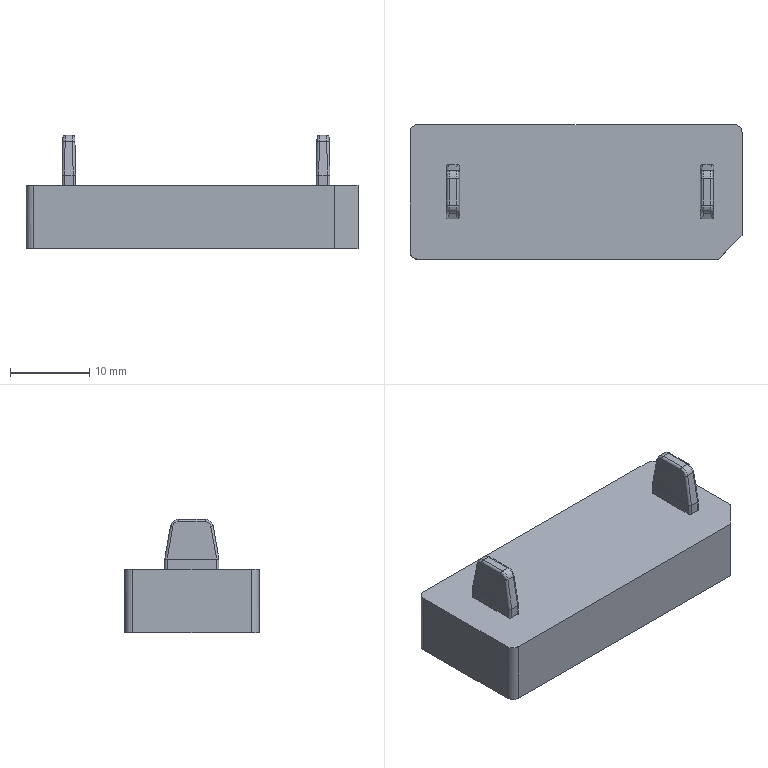NC program | PowerMill | posted by the shop | part box 42 x 17 x 14.346 mm
Lines 32786 to 34275 of 86217:
( TOOL ID   B4R0.5_1_1 )
( TOOL DIA. 4. TIP RAD .5 LENGTH 61.52 )
( Z = -6.52 )
T5 M6
T13
G91 G28 Z0
G0 G90 G54
M08
S18000 M3
X0 Y0 M8
G43 Z10.796 H5
X18.342 Y-3.827
Z.917
G1 Z-.283 F1200
X18.325 Y-3.779 F2000
X18.304 Y-3.733
X18.28 Y-3.689
X18.253 Y-3.646
X18.222 Y-3.606
X18.188 Y-3.569
X18.151 Y-3.534
X18.112 Y-3.503
X18.07 Y-3.474
X18.026 Y-3.449
X17.98 Y-3.427
X17.933 Y-3.41
X17.885 Y-3.396
X17.835 Y-3.385
X17.785 Y-3.379
X17.734 Y-3.377
X17.684 Y-3.378
X17.634 Y-3.384
X17.584 Y-3.394
X17.541 Y-3.406
X17.486 Y-3.423
X17.429 Y-3.438
X17.373 Y-3.451
X17.316 Y-3.462
X17.255 Y-3.471
X17.194 Y-3.478
X17.133 Y-3.483
X17.07 Y-3.486
X17.008 Y-3.487
X16.947
X16.885 Y-3.486
X16.823
X16.631
X16.509 Y-3.487
X16.405 Y-3.486
X16.291
X16.047 Y-3.485
X16.009 Y-3.483
X15.972 Y-3.479
X15.924 Y-3.474
X15.887 Y-3.469
X15.849 Y-3.463
X15.812 Y-3.456
X15.743 Y-3.441
X15.69 Y-3.427
X15.61 Y-3.403
X15.53 Y-3.373
X15.451 Y-3.341
X15.377 Y-3.306
X15.307 Y-3.269
X15.243 Y-3.231
X15.184 Y-3.192
X15.13 Y-3.153
X15.077 Y-3.112
X15.025 Y-3.07
X14.975 Y-3.025
X14.928 Y-2.979
X14.883 Y-2.93
X14.839 Y-2.879
X14.798 Y-2.827
X14.758 Y-2.773
X14.711 Y-2.706
X14.668 Y-2.636
X14.628 Y-2.565
X14.591 Y-2.491
X14.558 Y-2.416
X14.528 Y-2.338
X14.501 Y-2.257
X14.477 Y-2.174
X14.457 Y-2.088
X14.44 Y-1.999
X14.429 Y-1.93
X14.421 Y-1.86
X14.417 Y-1.78
X14.414 Y-1.685
Y-1.558
Y1.194
Y1.558
Y1.623
Y1.688
X14.415 Y1.752
X14.417 Y1.821
X14.422 Y1.9
X14.429 Y1.972
X14.438 Y2.036
X14.45 Y2.099
X14.464 Y2.162
X14.48 Y2.224
X14.498 Y2.286
X14.519 Y2.351
X14.542 Y2.416
X14.568 Y2.479
X14.597 Y2.541
X14.628 Y2.602
X14.66 Y2.662
X14.695 Y2.721
X14.736 Y2.784
X14.782 Y2.847
X14.834 Y2.912
X14.892 Y2.978
X14.947 Y3.036
X15.006 Y3.091
X15.068 Y3.144
X15.132 Y3.195
X15.2 Y3.242
X15.271 Y3.287
X15.345 Y3.329
X15.412 Y3.363
X15.483 Y3.395
X15.558 Y3.424
X15.637 Y3.45
X15.72 Y3.474
X15.809 Y3.495
X15.872 Y3.507
X15.94 Y3.516
X16.015 Y3.522
X16.1 Y3.525
X16.164 Y3.526
X16.509 Y3.525
X16.727 Y3.524
X16.97 Y3.525
X17.068
X17.144 Y3.522
X17.201 Y3.517
X17.252 Y3.511
X17.304 Y3.503
X17.354 Y3.494
X17.405 Y3.483
X17.455 Y3.47
X17.525 Y3.449
X17.595 Y3.426
X17.664 Y3.4
X17.731 Y3.372
X17.799 Y3.338
X17.869 Y3.299
X17.939 Y3.256
X18.009 Y3.209
X18.075 Y3.159
X18.137 Y3.108
X18.191 Y3.058
X18.243 Y3.006
X18.296 Y2.947
X18.352 Y2.88
X18.392 Y2.829
X18.427 Y2.779
X18.461 Y2.727
X18.492 Y2.674
X18.526 Y2.613
X18.563 Y2.54
X18.599 Y2.461
X18.628 Y2.39
X18.65 Y2.328
X18.668 Y2.269
X18.684 Y2.209
X18.705 Y2.115
X18.722 Y2.029
X18.733 Y1.95
X18.741 Y1.873
X18.745 Y1.792
X18.746 Y1.693
Y1.558
Y-.169
Y-1.443
X18.747 Y-1.607
X18.746 Y-1.72
X18.742 Y-1.813
X18.736 Y-1.894
X18.728 Y-1.961
X18.716 Y-2.028
X18.701 Y-2.102
X18.68 Y-2.184
X18.654 Y-2.271
X18.626 Y-2.353
X18.597 Y-2.427
X18.568 Y-2.493
X18.538 Y-2.554
X18.505 Y-2.613
X18.457 Y-2.692
X18.409 Y-2.764
X18.36 Y-2.831
X18.31 Y-2.892
X18.26 Y-2.949
X18.207 Y-3.002
X18.144 Y-3.061
X18.081 Y-3.114
X18.018 Y-3.163
X17.955 Y-3.207
X17.891 Y-3.246
X17.815 Y-3.289
X17.738 Y-3.327
X17.66 Y-3.361
X17.581 Y-3.392
X17.541 Y-3.406
X17.476 Y-3.427 Z-.284
X17.407 Y-3.445
X17.334 Y-3.461
X17.269 Y-3.472
X17.202 Y-3.481
X17.137 Y-3.487
X17.072 Y-3.49
X16.924 Y-3.491
X16.63 Y-3.492 Z-.285
X16.393 Y-3.495
X16.214 Y-3.496 Z-.286
X16.045 Y-3.494
X15.977 Y-3.491
X15.907 Y-3.484
X15.834 Y-3.473
X15.758 Y-3.458
X15.679 Y-3.438 Z-.287
X15.599 Y-3.413
X15.52 Y-3.386
X15.444 Y-3.354
X15.37 Y-3.32
X15.298 Y-3.282
X15.227 Y-3.24 Z-.288
X15.166 Y-3.2
X15.108 Y-3.159
X15.052 Y-3.114
X14.992 Y-3.062
X14.931 Y-3.005
X14.88 Y-2.952
X14.832 Y-2.899 Z-.289
X14.787 Y-2.844
X14.735 Y-2.775
X14.687 Y-2.704
X14.643 Y-2.631
X14.602 Y-2.557 Z-.29
X14.565 Y-2.482
X14.532 Y-2.406
X14.508 Y-2.344
X14.486 Y-2.281
X14.466 Y-2.218
X14.449 Y-2.154 Z-.291
X14.434 Y-2.089
X14.421 Y-2.024
X14.41 Y-1.959
X14.399 Y-1.879
X14.392 Y-1.798 Z-.292
X14.389 Y-1.715
Y-1.631
X14.382 Y-.215 Z-.295
X14.374 Y1.283 Z-.298
X14.372 Y1.617
Y1.741 Z-.299
X14.373 Y1.83
X14.378 Y1.904
X14.387 Y1.989
X14.4 Y2.074
X14.417 Y2.161
X14.439 Y2.249 Z-.3
X14.465 Y2.338
X14.492 Y2.419
X14.522 Y2.496
X14.554 Y2.57
X14.589 Y2.64
X14.63 Y2.713
X14.675 Y2.787
X14.724 Y2.859 Z-.301
X14.775 Y2.928
X14.827 Y2.992
X14.88 Y3.05
X14.933 Y3.104
X14.985 Y3.153
X15.04 Y3.2
X15.096 Y3.245
X15.154 Y3.288
X15.214 Y3.328
X15.282 Y3.369 Z-.302
X15.352 Y3.407
X15.425 Y3.443
X15.5 Y3.475
X15.578 Y3.504
X15.659 Y3.53
X15.727 Y3.549
X15.795 Y3.565 Z-.303
X15.863 Y3.579
X15.932 Y3.589
X16.002 Y3.596
X16.072 Y3.6
X16.142 Y3.601
X16.212
X16.52 Y3.603 Z-.304
X16.827 Y3.606 Z-.305
X17.087 Y3.607
X17.15 Y3.605
X17.219 Y3.599
X17.293 Y3.589 Z-.306
X17.375 Y3.574
X17.449 Y3.558
X17.524 Y3.537
X17.601 Y3.512
X17.681 Y3.483 Z-.307
X17.759 Y3.45
X17.823 Y3.419
X17.887 Y3.384
X17.955 Y3.344
X18.025 Y3.297 Z-.308
X18.094 Y3.247
X18.158 Y3.196
X18.214 Y3.147
X18.266 Y3.097 Z-.309
X18.324 Y3.036
X18.38 Y2.972
X18.432 Y2.906
X18.481 Y2.838
X18.527 Y2.767 Z-.31
X18.569 Y2.694
X18.612 Y2.614
X18.649 Y2.534
X18.682 Y2.455
X18.711 Y2.377 Z-.311
X18.736 Y2.297
X18.759 Y2.211
X18.779 Y2.122
X18.795 Y2.031
X18.807 Y1.939
X18.815 Y1.844 Z-.312
X18.82 Y1.748
X18.821 Y1.65
X18.822 Y1.154 Z-.313
X18.826 Y.432 Z-.314
X18.828 Y-.229 Z-.316
X18.834 Y-1.559 Z-.318
X18.835 Y-1.642 Z-.319
X18.833 Y-1.752
X18.829 Y-1.843
X18.822 Y-1.926
X18.81 Y-2.016
X18.794 Y-2.105
X18.774 Y-2.194 Z-.32
X18.751 Y-2.281
X18.724 Y-2.367
X18.693 Y-2.451
X18.658 Y-2.534
X18.62 Y-2.615 Z-.321
X18.579 Y-2.693
X18.534 Y-2.769
X18.486 Y-2.843
X18.445 Y-2.901
X18.401 Y-2.957
X18.351 Y-3.017 Z-.322
X18.293 Y-3.079
X18.23 Y-3.142
X18.169 Y-3.198
X18.11 Y-3.247
X18.053 Y-3.29
X17.996 Y-3.329
X17.922 Y-3.376 Z-.323
X17.847 Y-3.419
X17.775 Y-3.456
X17.705 Y-3.487
X17.638 Y-3.514
X17.582 Y-3.532
X17.508 Y-3.557 Z-.324
X17.431 Y-3.579
X17.353 Y-3.596
X17.276 Y-3.61
X17.201 Y-3.619
X17.129 Y-3.625
X17.058 Y-3.626
X16.967 Y-3.627 Z-.325
X16.875 Y-3.628
X16.784 Y-3.629
X16.693 Y-3.63
X16.566 Y-3.631
X16.475 Y-3.632
X16.384 Z-.326
X16.293 Y-3.633
X16.202
X16.111 Y-3.632
X16.036 Y-3.631
X15.961 Y-3.626
X15.887 Y-3.618 Z-.327
X15.811 Y-3.606
X15.733 Y-3.589
X15.653 Y-3.568
X15.569 Y-3.542
X15.498 Y-3.517
X15.426 Y-3.488 Z-.328
X15.353 Y-3.454
X15.283 Y-3.418
X15.217 Y-3.381
X15.152 Y-3.34
X15.086 Y-3.294
X15.02 Y-3.243 Z-.329
X14.952 Y-3.186
X14.894 Y-3.133
X14.838 Y-3.076
X14.782 Y-3.014
X14.727 Y-2.948
X14.675 Y-2.878 Z-.33
X14.625 Y-2.805
X14.578 Y-2.729
X14.536 Y-2.654
X14.498 Y-2.579
X14.465 Y-2.505
X14.436 Y-2.431
X14.412 Y-2.366 Z-.331
X14.391 Y-2.301
X14.366 Y-2.211
X14.346 Y-2.129
X14.331 Y-2.052
X14.32 Y-1.978
X14.311 Y-1.894 Z-.332
X14.304 Y-1.81
X14.301 Y-1.726
X14.299 Y-1.642
Y-1.557
Y-1.473
X14.296 Y-.71 Z-.334
X14.292 Y.46 Z-.336
X14.287 Y1.623 Z-.338
Y1.698
X14.289 Y1.806 Z-.339
X14.293 Y1.894
X14.299 Y1.972
X14.309 Y2.046
X14.326 Y2.143
X14.346 Y2.237 Z-.34
X14.37 Y2.328
X14.396 Y2.414
X14.426 Y2.498
X14.46 Y2.581
X14.497 Y2.663
X14.538 Y2.742 Z-.341
X14.582 Y2.82
X14.629 Y2.895
X14.68 Y2.968
X14.734 Y3.039
X14.792 Y3.107
X14.84 Y3.16 Z-.342
X14.89 Y3.21
X14.947 Y3.262
X15.013 Y3.318
X15.071 Y3.363
X15.128 Y3.405
X15.188 Y3.444
X15.26 Y3.487 Z-.343
X15.335 Y3.527
X15.411 Y3.563
X15.49 Y3.597
X15.571 Y3.626
X15.653 Y3.652
X15.737 Y3.674 Z-.344
X15.818 Y3.692
X15.895 Y3.706
X15.967 Y3.715
X16.036 Y3.719
X16.104 Y3.721
X16.197 Y3.722
X16.29 Y3.723 Z-.345
X16.382 Y3.724
X16.475
X16.596 Y3.725
X16.688
X16.781 Z-.346
X16.874
X16.966
X17.059
X17.126
X17.195 Y3.72
X17.268 Y3.712 Z-.347
X17.345 Y3.699
X17.428 Y3.681
X17.52 Y3.657
X17.587 Y3.638
X17.656 Y3.614
X17.729 Y3.584
X17.806 Y3.55 Z-.348
X17.883 Y3.511
X17.957 Y3.469
X18.025 Y3.426
X18.086 Y3.384
X18.144 Y3.339
X18.209 Y3.286 Z-.349
X18.272 Y3.228
X18.335 Y3.166
X18.395 Y3.101
X18.451 Y3.034
X18.503 Y2.967
X18.55 Y2.9 Z-.35
X18.593 Y2.83
X18.638 Y2.753
X18.679 Y2.672
X18.718 Y2.589
X18.753 Y2.502
X18.783 Y2.42 Z-.351
X18.81 Y2.336
X18.833 Y2.249
X18.852 Y2.16
X18.869 Y2.067
X18.881 Y1.973
X18.89 Y1.875 Z-.352
X18.896 Y1.774
X18.898 Y1.674
X18.899 Y1.011 Z-.353
X18.902 Y.067 Z-.355
X18.905 Y-.823 Z-.357
X18.908 Y-1.675 Z-.359
X18.906 Y-1.772
X18.9 Y-1.869
X18.891 Y-1.964
X18.878 Y-2.059
X18.86 Y-2.152
X18.84 Y-2.243 Z-.36
X18.815 Y-2.332
X18.787 Y-2.42
X18.755 Y-2.506
X18.72 Y-2.591
X18.681 Y-2.673 Z-.361
X18.639 Y-2.753
X18.594 Y-2.831
X18.546 Y-2.906
X18.494 Y-2.979
X18.44 Y-3.048
X18.384 Y-3.114 Z-.362
X18.325 Y-3.177
X18.263 Y-3.237
X18.198 Y-3.295
X18.131 Y-3.349
X18.061 Y-3.4
X17.99 Y-3.448 Z-.363
X17.916 Y-3.492
X17.841 Y-3.532
X17.765 Y-3.569
X17.687 Y-3.602
X17.616 Y-3.628
X17.53 Y-3.656 Z-.364
X17.447 Y-3.679
X17.367 Y-3.698
X17.292 Y-3.711
X17.215 Y-3.721
X17.133 Y-3.728
X17.044 Y-3.731
X16.947 Z-.365
X16.751
X16.484 Y-3.733 Z-.366
X16.196 Y-3.735
X16.117
X16.038 Y-3.733
X15.96 Y-3.727 Z-.367
X15.88 Y-3.718
X15.8 Y-3.705
X15.723 Y-3.689
X15.646 Y-3.669
X15.571 Y-3.646
X15.492 Y-3.619
X15.414 Y-3.588 Z-.368
X15.338 Y-3.554
X15.265 Y-3.516
X15.195 Y-3.476
X15.126 Y-3.433
X15.057 Y-3.386
X14.991 Y-3.335 Z-.369
X14.926 Y-3.281
X14.864 Y-3.225
X14.805 Y-3.166
X14.759 Y-3.117
X14.715 Y-3.066
X14.673 Y-3.013
X14.627 Y-2.95 Z-.37
X14.577 Y-2.877
X14.539 Y-2.817
X14.504 Y-2.759
X14.472 Y-2.699
X14.433 Y-2.616
X14.396 Y-2.532
X14.363 Y-2.446 Z-.371
X14.334 Y-2.358
X14.308 Y-2.269
X14.286 Y-2.178
X14.268 Y-2.086
X14.253 Y-1.993
X14.242 Y-1.898 Z-.372
X14.235 Y-1.801
X14.232 Y-1.703
Y-1.603
X14.228 Y-.402 Z-.374
X14.226 Y.785 Z-.377
X14.223 Y1.51 Z-.378
X14.222 Y1.674
X14.223 Y1.771 Z-.379
X14.227 Y1.874
X14.235 Y1.974
X14.247 Y2.069
X14.261 Y2.158
X14.278 Y2.242
X14.299 Y2.325 Z-.38
X14.325 Y2.417
X14.355 Y2.505
X14.387 Y2.592
X14.423 Y2.675
X14.463 Y2.757
X14.505 Y2.836 Z-.381
X14.551 Y2.914
X14.6 Y2.988
X14.652 Y3.06
X14.707 Y3.13
X14.765 Y3.196
X14.825 Y3.26 Z-.382
X14.888 Y3.321
X14.953 Y3.378
X15.021 Y3.433
X15.091 Y3.484
X15.163 Y3.531
X15.236 Y3.575 Z-.383
X15.312 Y3.615
X15.388 Y3.651
X15.466 Y3.685
X15.548 Y3.714
X15.631 Y3.741
X15.715 Y3.763 Z-.384
X15.8 Y3.782
X15.885 Y3.797
X15.969 Y3.807
X16.052 Y3.814
X16.134 Y3.816
X16.215 Y3.815 Z-.385
X16.502 Y3.814
X16.79 Y3.816 Z-.386
X17.007 Y3.818
X17.095 Y3.817
X17.18 Y3.813
X17.261 Y3.805 Z-.387
X17.34 Y3.793
X17.416 Y3.778
X17.491 Y3.759
X17.578 Y3.734
X17.662 Y3.705
X17.745 Y3.673
X17.814 Y3.642 Z-.388
X17.882 Y3.609
X17.952 Y3.57
X18.026 Y3.524
X18.1 Y3.475
X18.167 Y3.426
X18.226 Y3.379 Z-.389
X18.283 Y3.329
X18.345 Y3.269
X18.405 Y3.206
X18.463 Y3.139
X18.519 Y3.069
X18.572 Y2.995 Z-.39
X18.622 Y2.919
X18.669 Y2.841
X18.713 Y2.761
X18.752 Y2.68
X18.787 Y2.598
X18.821 Y2.51 Z-.391
X18.851 Y2.42
X18.877 Y2.329
X18.9 Y2.236
X18.919 Y2.142
X18.934 Y2.046
X18.945 Y1.956 Z-.392
X18.952 Y1.861
X18.956 Y1.757
X18.957 Y1.642
X18.959 Y.667 Z-.394
X18.964 Y-1.001 Z-.397
X18.966 Y-1.676 Z-.398
X18.964 Y-1.774 Z-.399
X18.959 Y-1.873
X18.949 Y-1.972
X18.936 Y-2.069
X18.918 Y-2.166
X18.898 Y-2.26 Z-.4
X18.873 Y-2.352
X18.845 Y-2.442
X18.814 Y-2.529
X18.78 Y-2.614
X18.741 Y-2.699
X18.699 Y-2.782 Z-.401
X18.654 Y-2.862
X18.607 Y-2.939
X18.556 Y-3.013
X18.502 Y-3.084
X18.446 Y-3.153
X18.387 Y-3.218 Z-.402
X18.325 Y-3.282
X18.259 Y-3.342
X18.196 Y-3.396
X18.129 Y-3.448
X18.058 Y-3.498
X17.985 Y-3.545 Z-.403
X17.91 Y-3.588
X17.834 Y-3.627
X17.759 Y-3.661
X17.685 Y-3.691
X17.641 Y-3.707
X17.552 Y-3.736 Z-.404
X17.467 Y-3.76
X17.388 Y-3.78
X17.311 Y-3.795
X17.238 Y-3.805
X17.165 Y-3.811
X17.093 Y-3.814
X17.02 Y-3.815 Z-.405
X16.636 Y-3.816
X16.252 Y-3.818 Z-.406
X16.162 Y-3.819
X16.086
X16.01 Y-3.816
X15.934 Y-3.81 Z-.407
X15.859 Y-3.8
X15.784 Y-3.787
X15.704 Y-3.769
X15.63 Y-3.749
X15.557 Y-3.728
X15.476 Y-3.7
X15.397 Y-3.669 Z-.408
X15.321 Y-3.634
X15.247 Y-3.597
X15.176 Y-3.556
X15.107 Y-3.512
X15.032 Y-3.461
X14.961 Y-3.407
X14.893 Y-3.35 Z-.409
X14.828 Y-3.291
X14.767 Y-3.23
X14.71 Y-3.167
X14.653 Y-3.098
X14.598 Y-3.027
X14.547 Y-2.953 Z-.41
X14.498 Y-2.876
X14.453 Y-2.796
X14.41 Y-2.714
X14.371 Y-2.63
X14.336 Y-2.543
X14.303 Y-2.454 Z-.411
X14.275 Y-2.364
X14.249 Y-2.271
X14.228 Y-2.177
X14.21 Y-2.081
X14.196 Y-1.983 Z-.412
X14.186 Y-1.884
X14.179 Y-1.783
X14.177 Y-1.681
Y-1.578
X14.173 Y.002 Z-.415
X14.171 Y1.24 Z-.418
X14.17 Y1.674
X14.171 Y1.785 Z-.419
X14.176 Y1.891
X14.184 Y1.992
X14.196 Y2.09
X14.212 Y2.184
X14.23 Y2.277
X14.252 Y2.366 Z-.42
X14.279 Y2.459
X14.309 Y2.548
X14.342 Y2.636
X14.379 Y2.721
X14.419 Y2.804
X14.462 Y2.884 Z-.421
X14.508 Y2.963
X14.558 Y3.039
X14.609 Y3.111
X14.664 Y3.182
X14.722 Y3.25
X14.784 Y3.316 Z-.422
X14.848 Y3.378
X14.914 Y3.438
X14.982 Y3.493
X15.046 Y3.541
X15.116 Y3.589
X15.19 Y3.635 Z-.423
X15.266 Y3.677
X15.34 Y3.713
X15.411 Y3.745
X15.482 Y3.772
X15.547 Y3.794
X15.612 Y3.815
X15.678 Y3.833 Z-.424
X15.708 Y3.842
X15.737 Y3.849
X15.767 Y3.855
X15.802 Y3.862
X15.85 Y3.871
X15.88 Y3.876
X15.91 Y3.88
X15.94 Y3.884
X16.03 Y3.889
X16.134 Y3.892
X16.273 Y3.893 Z-.425
X16.555 Y3.894
X16.97 Y3.896 Z-.426
X17.038
X17.106 Y3.895
X17.174 Y3.892
X17.242 Y3.886
X17.31 Y3.877 Z-.427
X17.377 Y3.864
X17.443 Y3.849
X17.509 Y3.832
X17.575 Y3.814
X17.652 Y3.79
X17.73 Y3.76
X17.809 Y3.726 Z-.428
X17.882 Y3.691
X17.959 Y3.65
X18.033 Y3.606
X18.105 Y3.559
X18.174 Y3.509
X18.241 Y3.456 Z-.429
X18.309 Y3.396
X18.374 Y3.334
X18.435 Y3.27
X18.493 Y3.204
X18.548 Y3.136
X18.599 Y3.066
X18.65 Y2.989 Z-.43
X18.698 Y2.911
X18.742 Y2.831
X18.783 Y2.748
X18.821 Y2.664
X18.855 Y2.577 Z-.431
X18.886 Y2.488
X18.914 Y2.398
X18.938 Y2.305
X18.959 Y2.21
X18.976 Y2.113
X18.989 Y2.013 Z-.432
X18.999 Y1.911
X19.005 Y1.807
X19.008 Y1.7
X19.007 Y1.589
Y1.07 Z-.433
X19.01 Y.304 Z-.435
Y-.368 Z-.436
X19.013 Y-1.297 Z-.438
X19.014 Y-1.559
Y-1.697
X19.011 Y-1.806 Z-.439
X19.005 Y-1.899
X18.996 Y-1.992
X18.983 Y-2.091
X18.965 Y-2.188
X18.944 Y-2.285 Z-.44
X18.919 Y-2.379
X18.89 Y-2.472
X18.858 Y-2.563
X18.823 Y-2.652
X18.784 Y-2.738
X18.742 Y-2.822 Z-.441
X18.697 Y-2.903
X18.649 Y-2.982
X18.598 Y-3.057
X18.544 Y-3.13
X18.488 Y-3.199
X18.429 Y-3.266 Z-.442
X18.366 Y-3.331
X18.301 Y-3.392
X18.234 Y-3.45
X18.164 Y-3.505
X18.092 Y-3.556
X18.019 Y-3.604 Z-.443
X17.944 Y-3.648
X17.868 Y-3.688
X17.791 Y-3.724
X17.713 Y-3.756
X17.666 Y-3.774
X17.589 Y-3.8
X17.511 Y-3.823 Z-.444
X17.43 Y-3.843
X17.348 Y-3.86
X17.264 Y-3.873
X17.182 Y-3.883
X17.101 Y-3.888
X17.02 Y-3.891 Z-.445
X16.939
X16.589 Y-3.89
X16.165 Y-3.893 Z-.446
X16.081 Y-3.892
X15.996 Y-3.887
X15.911 Y-3.879 Z-.447
X15.826 Y-3.867
X15.743 Y-3.851
X15.66 Y-3.831
X15.574 Y-3.807
X15.49 Y-3.78
X15.408 Y-3.749
X15.33 Y-3.715 Z-.448
X15.254 Y-3.677
X15.18 Y-3.637
X15.105 Y-3.591
X15.032 Y-3.542
X14.961 Y-3.49
X14.892 Y-3.434 Z-.449
X14.825 Y-3.375
X14.762 Y-3.314
X14.702 Y-3.25
X14.644 Y-3.182
X14.588 Y-3.111
X14.534 Y-3.037 Z-.45
X14.484 Y-2.96
X14.436 Y-2.88
X14.391 Y-2.798
X14.351 Y-2.713
X14.313 Y-2.628
X14.28 Y-2.541 Z-.451
X14.248 Y-2.449
X14.221 Y-2.355
X14.197 Y-2.259
X14.176 Y-2.163
X14.159 Y-2.064
X14.147 Y-1.964 Z-.452
X14.137 Y-1.862
X14.132 Y-1.759
X14.131 Y-1.653
X14.128 Y.001 Z-.455
X14.126 Y1.12 Z-.457
X14.124 Y1.674 Z-.458
X14.125 Y1.786
X14.13 Y1.895 Z-.459
X14.139 Y2.
X14.151 Y2.102
X14.167 Y2.2
X14.186 Y2.296
X14.21 Y2.392 Z-.46
X14.237 Y2.485
X14.267 Y2.577
X14.301 Y2.667
X14.334 Y2.745
X14.369 Y2.821
X14.407 Y2.896 Z-.461
X14.45 Y2.972
X14.495 Y3.044
X14.542 Y3.113
X14.591 Y3.18
X14.645 Y3.249
X14.702 Y3.315 Z-.462
X14.762 Y3.379
X14.824 Y3.439
X14.888 Y3.496
X14.954 Y3.55
X15.023 Y3.601
X15.094 Y3.649
X15.16 Y3.69 Z-.463
X15.229 Y3.729
X15.298 Y3.765
X15.371 Y3.799
X15.448 Y3.831
X15.526 Y3.859
X15.602 Y3.883
X15.678 Y3.904 Z-.464
X15.755 Y3.922
X15.835 Y3.938
X15.913 Y3.949
X15.987 Y3.956
X16.059 Y3.96
X16.159 Y3.961
X16.259 Y3.962 Z-.465
X16.359 Y3.963
X16.459
X16.579
X16.679 Y3.964
X16.778 Z-.466
X16.878
X16.978 Y3.965
X17.052
X17.126 Y3.963
X17.202 Y3.957
X17.282 Y3.948 Z-.467
X17.366 Y3.934
X17.454 Y3.915
X17.542 Y3.893
X17.629 Y3.867
X17.71 Y3.838
X17.785 Y3.809
X17.854 Y3.778 Z-.468
X17.92 Y3.745
X17.994 Y3.704
X18.068 Y3.658
X18.142 Y3.608
X18.214 Y3.554
X18.285 Y3.497 Z-.469
X18.352 Y3.437
X18.415 Y3.376
X18.474 Y3.313
X18.529 Y3.249
X18.585 Y3.178
X18.639 Y3.104 Z-.47
X18.69 Y3.027
X18.737 Y2.947
X18.782 Y2.864
X18.823 Y2.779
X18.862 Y2.692
X18.896 Y2.602 Z-.471
X18.928 Y2.511
X18.955 Y2.418
X18.979 Y2.325
X19. Y2.229
X19.017 Y2.131
X19.031 Y2.03 Z-.472
X19.041 Y1.927
X19.047 Y1.821
X19.05 Y1.712
Y1.601
Y.927 Z-.474
X19.052 Y.037 Z-.475
X19.053 Y-.826 Z-.477
X19.055 Y-1.675 Z-.478
X19.054 Y-1.781 Z-.479
X19.048 Y-1.885
X19.039 Y-1.989
X19.025 Y-2.091
X19.009 Y-2.191
X18.988 Y-2.289
X18.964 Y-2.385 Z-.48
X18.936 Y-2.48
X18.905 Y-2.572
X18.87 Y-2.662
X18.832 Y-2.75
X18.79 Y-2.835 Z-.481
X18.746 Y-2.919
X18.698 Y-2.999
X18.648 Y-3.077
X18.594 Y-3.152
X18.538 Y-3.224
X18.479 Y-3.293 Z-.482
X18.417 Y-3.359
X18.354 Y-3.421
X18.289 Y-3.479
X18.222 Y-3.534
X18.149 Y-3.589
X18.076 Y-3.639 Z-.483
X18.001 Y-3.685
X17.926 Y-3.727
X17.849 Y-3.765
X17.772 Y-3.8
X17.695 Y-3.83
X17.688 Y-3.832
X17.63 Y-3.853
X17.571 Y-3.872 Z-.484
X17.503 Y-3.891
X17.422 Y-3.911
X17.337 Y-3.928
X17.262 Y-3.939
X17.196 Y-3.947
X17.134 Y-3.951
X17.072 Y-3.953
X16.636 Y-3.954 Z-.485
X16.2 Y-3.956 Z-.486
X16.108
X16.017 Y-3.952
X15.929 Y-3.945
X15.842 Y-3.934 Z-.487
X15.758 Y-3.919
X15.675 Y-3.901
X15.593 Y-3.879
X15.513 Y-3.854
X15.428 Y-3.823
X15.347 Y-3.79 Z-.488
X15.271 Y-3.754
X15.197 Y-3.716
X15.121 Y-3.672
X15.046 Y-3.623
X14.973 Y-3.572
X14.902 Y-3.517
X14.835 Y-3.459 Z-.489
X14.77 Y-3.4
X14.71 Y-3.338
X14.653 Y-3.275
X14.595 Y-3.206
X14.542 Y-3.136
X14.49 Y-3.062 Z-.49
X14.44 Y-2.984
X14.393 Y-2.903
X14.349 Y-2.819
X14.308 Y-2.732
X14.274 Y-2.652
X14.244 Y-2.571 Z-.491
X14.215 Y-2.486
X14.188 Y-2.395
X14.166 Y-2.312
X14.147 Y-2.228
X14.131 Y-2.144
X14.118 Y-2.06 Z-.492
X14.108 Y-1.975
X14.1 Y-1.889
X14.094 Y-1.793
X14.092 Y-1.707
X14.091 Y-1.622
Y-1.536
X14.092 Y-1.45 Z-.493
X14.091 Y-1.028
X14.09 Y-.543 Z-.494
X14.089 Y.459 Z-.496
X14.087 Y1.462 Z-.498
X14.086 Y1.674
X14.087 Y1.789
X14.092 Y1.9 Z-.499
X14.101 Y2.008
X14.113 Y2.112
X14.129 Y2.213
X14.149 Y2.312
X14.172 Y2.408 Z-.5
X14.198 Y2.504
X14.229 Y2.598
X14.263 Y2.689
X14.3 Y2.779
X14.34 Y2.866
X14.384 Y2.95 Z-.501
X14.431 Y3.032
X14.48 Y3.11
X14.533 Y3.186
X14.588 Y3.26
X14.646 Y3.33
X14.707 Y3.397 Z-.502
X14.771 Y3.462
X14.837 Y3.523
X14.905 Y3.582
X14.976 Y3.636
X15.048 Y3.688
X15.123 Y3.736 Z-.503
X15.199 Y3.78
X15.277 Y3.82
X15.356 Y3.857
X15.434 Y3.889
X15.516 Y3.919
X15.603 Y3.946
X15.694 Y3.97 Z-.504
X15.775 Y3.988
X15.857 Y4.002
X15.943 Y4.013
X16.031 Y4.02
X16.123 Y4.023
X16.218 Z-.505
X16.761 Y4.024 Z-.506
X16.901 Y4.025
X16.983 Y4.026
X17.086 Y4.025
X17.172 Y4.021
X17.202 Y4.018
X17.233 Y4.015
X17.263 Y4.011
X17.299 Y4.006 Z-.507
X17.346 Y3.998
X17.376 Y3.993
X17.406 Y3.988
X17.436 Y3.981
X17.517 Y3.962
X17.593 Y3.941
X17.674 Y3.915
X17.755 Y3.884
X17.835 Y3.85 Z-.508
X17.914 Y3.812
X17.992 Y3.771
X18.068 Y3.725
X18.142 Y3.676
X18.215 Y3.623
X18.285 Y3.567
X18.352 Y3.509 Z-.509
X18.417 Y3.447
X18.48 Y3.382
X18.54 Y3.314
X18.597 Y3.243
X18.652 Y3.169
X18.704 Y3.092 Z-.51
X18.753 Y3.012
X18.799 Y2.929
X18.842 Y2.844
X18.881 Y2.756
X18.918 Y2.667
X18.95 Y2.575 Z-.511
X18.98 Y2.481
X19.004 Y2.39
X19.026 Y2.295
X19.045 Y2.198
X19.06 Y2.099 Z-.512
X19.072 Y1.995
X19.08 Y1.888
X19.085 Y1.778
X19.086 Y1.674
X19.087 Y.676 Z-.514
X19.089 Y-.472 Z-.516
X19.091 Y-1.676 Z-.518
X19.09 Y-1.778
X19.084 Y-1.883 Z-.519
X19.075 Y-1.99
X19.062 Y-2.096
X19.045 Y-2.198
X19.026 Y-2.295
X19.003 Y-2.387 Z-.52
X18.976 Y-2.483
X18.945 Y-2.578
X18.911 Y-2.67
X18.873 Y-2.76
X18.832 Y-2.848
X18.788 Y-2.933 Z-.521
X18.741 Y-3.015
X18.691 Y-3.094
X18.639 Y-3.171
X18.585 Y-3.242
X18.528 Y-3.311
X18.468 Y-3.378 Z-.522
X18.404 Y-3.443
X18.338 Y-3.505
X18.269 Y-3.564
X18.197 Y-3.62
X18.124 Y-3.672
X18.05 Y-3.72 Z-.523
X17.974 Y-3.764
X17.898 Y-3.804
X17.821 Y-3.84
X17.744 Y-3.871
X17.708 Y-3.885
X17.636 Y-3.911
X17.559 Y-3.935 Z-.524
X17.476 Y-3.957
X17.385 Y-3.977
X17.312 Y-3.99
X17.238 Y-4.
X17.164 Y-4.007
X17.081 Y-4.011
X17.006 Y-4.012 Z-.525
X16.932
X16.542 Y-4.011
X16.265 Y-4.012 Z-.526
X16.161 Y-4.014
X16.074 Y-4.013
X15.987 Y-4.008
X15.9 Y-4. Z-.527
X15.813 Y-3.987
X15.726 Y-3.971
X15.639 Y-3.95
X15.553 Y-3.926
X15.468 Y-3.897
X15.385 Y-3.866
X15.304 Y-3.831 Z-.528
X15.227 Y-3.793
X15.151 Y-3.752
X15.074 Y-3.705
X14.999 Y-3.655
X14.926 Y-3.601
X14.856 Y-3.545 Z-.529
X14.789 Y-3.485
X14.724 Y-3.423
X14.667 Y-3.363
X14.612 Y-3.301
X14.56 Y-3.237
X14.51 Y-3.171
X14.463 Y-3.103 Z-.53
X14.418 Y-3.033
X14.371 Y-2.952
X14.327 Y-2.869
X14.285 Y-2.782
X14.247 Y-2.693
X14.212 Y-2.602 Z-.531
X14.181 Y-2.508
X14.153 Y-2.411
X14.128 Y-2.312
X14.107 Y-2.211
X14.089 Y-2.109
X14.076 Y-2.005 Z-.532
X14.066 Y-1.899
X14.06 Y-1.791
X14.057 Y-1.681
Y-1.569
X14.055 Y0 Z-.535
X14.054 Y.881 Z-.537
X14.052 Y1.674 Z-.538
X14.054 Y1.789
X14.059 Y1.902 Z-.539
X14.067 Y2.013
X14.08 Y2.12
X14.095 Y2.224
X14.114 Y2.324
X14.137 Y2.419 Z-.54
X14.162 Y2.512
X14.192 Y2.608
X14.226 Y2.702
X14.263 Y2.793
X14.303 Y2.882
X14.346 Y2.968 Z-.541
X14.393 Y3.051
X14.442 Y3.131
X14.493 Y3.208
X14.548 Y3.282
X14.606 Y3.354
X14.667 Y3.423 Z-.542
X14.73 Y3.489
X14.796 Y3.552
X14.865 Y3.612
X14.935 Y3.669
X15.007 Y3.721
X15.082 Y3.771
X15.156 Y3.816 Z-.543
X15.233 Y3.857
X15.312 Y3.896
X15.394 Y3.931
X15.478 Y3.962
X15.563 Y3.991
X15.651 Y4.015 Z-.544
X15.739 Y4.036
X15.826 Y4.052
X15.907 Y4.064
X15.983 Y4.072
X16.057 Y4.075
X16.153 Y4.077
X16.249 Y4.078 Z-.545
X16.344 Y4.079
X16.44
X16.543
X16.639
X16.735 Z-.546
X16.83
X16.926
X17.022
X17.097 Y4.078
X17.172 Y4.075
X17.249 Y4.068
X17.33 Y4.057 Z-.547
X17.415 Y4.041
X17.496 Y4.022
X17.578 Y4.001
X17.661 Y3.975
X17.742 Y3.946
X17.819 Y3.915
X17.894 Y3.88 Z-.548
X17.968 Y3.842
X18.044 Y3.799
X18.119 Y3.752
X18.193 Y3.702
X18.264 Y3.648
X18.333 Y3.59 Z-.549
X18.4 Y3.529
X18.465 Y3.465
X18.527 Y3.398
X18.587 Y3.328
X18.644 Y3.255
X18.697 Y3.179 Z-.55
X18.748 Y3.1
X18.796 Y3.019
X18.841 Y2.935
X18.883 Y2.848
X18.922 Y2.759
X18.957 Y2.667 Z-.551
X18.989 Y2.573
X19.018 Y2.477
X19.043 Y2.379
X19.065 Y2.277
X19.082 Y2.175
X19.097 Y2.07 Z-.552
X19.107 Y1.963
X19.115 Y1.852
X19.118 Y1.737
Y1.619
Y.981 Z-.554
X19.12 Y.1 Z-.555
Y-.72 Z-.557
X19.122 Y-1.501 Z-.558
X19.123 Y-1.632
X19.122 Y-1.739
X19.117 Y-1.852 Z-.559
X19.109 Y-1.965
X19.098 Y-2.071
X19.083 Y-2.17
X19.067 Y-2.26
X19.045 Y-2.362
X19.019 Y-2.462 Z-.56
X18.99 Y-2.558
X18.957 Y-2.653
X18.921 Y-2.744
X18.882 Y-2.833
X18.84 Y-2.92 Z-.561
X18.795 Y-3.003
X18.747 Y-3.084
X18.696 Y-3.163
X18.641 Y-3.239
X18.584 Y-3.312
X18.524 Y-3.382 Z-.562
X18.464 Y-3.447
X18.401 Y-3.509
X18.335 Y-3.57
X18.265 Y-3.628
X18.193 Y-3.683
X18.119 Y-3.734
X18.043 Y-3.781 Z-.563
X17.968 Y-3.824
X17.891 Y-3.863
X17.816 Y-3.898
X17.74 Y-3.928
X17.726 Y-3.933
X17.667 Y-3.955
X17.607 Y-3.975
X17.539 Y-3.995 Z-.564
X17.459 Y-4.015
X17.369 Y-4.033
X17.29 Y-4.047
X17.221 Y-4.055
X17.159 Y-4.061
X17.096 Y-4.064
X17.033
X16.43 Y-4.065 Z-.566
X16.162 Y-4.066
X16.066 Y-4.065
X15.976 Y-4.06
X15.891 Y-4.052
X15.807 Y-4.04 Z-.567
X15.722 Y-4.023
X15.636 Y-4.003
X15.549 Y-3.978
X15.462 Y-3.949
X15.375 Y-3.916
X15.301 Y-3.884 Z-.568
X15.225 Y-3.848
X15.147 Y-3.805
X15.072 Y-3.761
X15. Y-3.714
X14.928 Y-3.662
X14.857 Y-3.606
X14.788 Y-3.547 Z-.569
X14.722 Y-3.484
X14.658 Y-3.418
X14.597 Y-3.35
X14.538 Y-3.278
X14.482 Y-3.203
X14.43 Y-3.126 Z-.57
X14.38 Y-3.047
X14.333 Y-2.964
X14.289 Y-2.878
X14.249 Y-2.79
X14.211 Y-2.7
X14.177 Y-2.607 Z-.571
X14.147 Y-2.512
X14.119 Y-2.414
X14.095 Y-2.313
X14.075 Y-2.211
X14.058 Y-2.106 Z-.572
X14.044 Y-1.999
X14.035 Y-1.891
X14.029 Y-1.78
X14.028 Y-1.674
X14.026 Y-.372 Z-.575
X14.025 Y1.15 Z-.577
X14.024 Y1.674 Z-.578
X14.025 Y1.8
X14.03 Y1.917 Z-.579
X14.039 Y2.027
X14.05 Y2.131
X14.065 Y2.23
X14.083 Y2.327
X14.106 Y2.429
X14.133 Y2.528 Z-.58
X14.162 Y2.626
X14.196 Y2.72
X14.232 Y2.812
X14.272 Y2.901
X14.314 Y2.987 Z-.581
X14.36 Y3.071
X14.408 Y3.152
X14.46 Y3.23
X14.515 Y3.306
X14.572 Y3.379
X14.633 Y3.45
X14.697 Y3.517 Z-.582
X14.76 Y3.579
X14.826 Y3.639
X14.897 Y3.696
X14.97 Y3.751
X15.045 Y3.802
X15.121 Y3.85 Z-.583
X15.199 Y3.893
X15.277 Y3.933
X15.356 Y3.968
X15.438 Y4.
X15.522 Y4.029
X15.609 Y4.055 Z-.584
X15.695 Y4.077
X15.777 Y4.094
X15.859 Y4.108
X15.943 Y4.118
X16.027 Y4.125